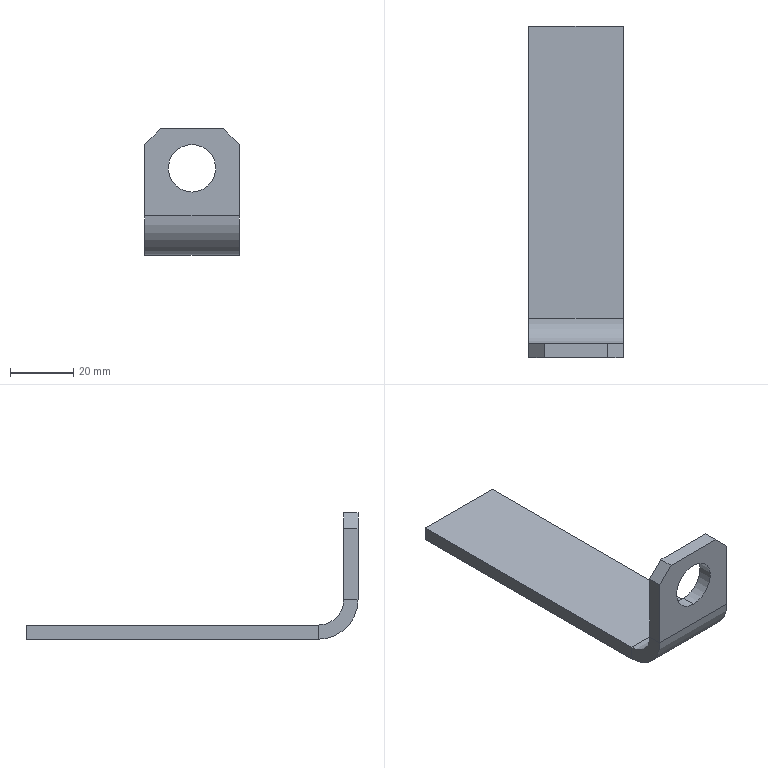Part | SolidWorks | features Chamfer 1, FlatPattern 1, ICE 1, SMBaseFlange 1, SheetMetal 1 | 1 solid | 18 faces | box 30 x 105 x 40 mm | volume 17466 mm3 | plane 14 | cylinder 4 | commonest cylinder face diameters 15 x2 16 x1 25 x1
STEP:
#1=CARTESIAN_POINT('',(0.,0.,-5.));
#2=VERTEX_POINT('',#1);
#3=CARTESIAN_POINT('',(0.,0.,-20.));
#4=VERTEX_POINT('',#3);
#5=CARTESIAN_POINT('',(0.,0.,-12.5));
#6=DIRECTION('',(0.,-1.,0.));
#7=DIRECTION('',(0.,0.,1.));
#8=AXIS2_PLACEMENT_3D('',#5,#6,#7);
#9=CIRCLE('',#8,7.5);
#10=EDGE_CURVE('',#2,#4,#9,.T.);
#11=ORIENTED_EDGE('',*,*,#10,.T.);
#12=CARTESIAN_POINT('',(0.,4.5,-20.));
#13=VERTEX_POINT('',#12);
#14=CARTESIAN_POINT('',(0.,-0.001,-20.));
#15=DIRECTION('',(0.,1.,0.));
#16=VECTOR('',#15,1000.);
#17=LINE('',#14,#16);
#18=EDGE_CURVE('',#4,#13,#17,.T.);
#19=ORIENTED_EDGE('',*,*,#18,.T.);
#20=CARTESIAN_POINT('',(0.,4.5,-5.));
#21=VERTEX_POINT('',#20);
#22=CARTESIAN_POINT('',(0.,4.5,-12.5));
#23=DIRECTION('',(0.,1.,0.));
#24=DIRECTION('',(0.,0.,1.));
#25=AXIS2_PLACEMENT_3D('',#22,#23,#24);
#26=CIRCLE('',#25,7.5);
#27=EDGE_CURVE('',#13,#21,#26,.T.);
#28=ORIENTED_EDGE('',*,*,#27,.T.);
#29=CARTESIAN_POINT('',(0.,-0.001,-5.));
#30=DIRECTION('',(0.,1.,0.));
#31=VECTOR('',#30,1000.);
#32=LINE('',#29,#31);
#33=EDGE_CURVE('',#2,#21,#32,.T.);
#34=ORIENTED_EDGE('',*,*,#33,.F.);
#35=EDGE_LOOP('',(#11,#19,#28,#34));
#36=FACE_OUTER_BOUND('',#35,.T.);
#37=CARTESIAN_POINT('',(0.,-0.001,-12.5));
#38=DIRECTION('',(0.,1.,0.));
#39=DIRECTION('',(0.,0.,1.));
#40=AXIS2_PLACEMENT_3D('',#37,#38,#39);
#41=CYLINDRICAL_SURFACE('',#40,7.5);
#42=ADVANCED_FACE('',(#36),#41,.F.);
#43=CARTESIAN_POINT('',(15.,0.,-27.5));
#44=VERTEX_POINT('',#43);
#45=CARTESIAN_POINT('',(15.,4.5,-27.5));
#46=VERTEX_POINT('',#45);
#47=CARTESIAN_POINT('',(15.,0.,-27.5));
#48=DIRECTION('',(0.,1.,0.));
#49=VECTOR('',#48,1000.);
#50=LINE('',#47,#49);
#51=EDGE_CURVE('',#44,#46,#50,.T.);
#52=ORIENTED_EDGE('',*,*,#51,.F.);
#53=CARTESIAN_POINT('',(15.,12.5,-40.));
#54=VERTEX_POINT('',#53);
#55=CARTESIAN_POINT('',(15.,12.5,-27.5));
#56=DIRECTION('',(1.,0.,0.));
#57=DIRECTION('',(0.,0.,1.));
#58=AXIS2_PLACEMENT_3D('',#55,#56,#57);
#59=CIRCLE('',#58,12.5);
#60=EDGE_CURVE('',#44,#54,#59,.T.);
#61=ORIENTED_EDGE('',*,*,#60,.T.);
#62=CARTESIAN_POINT('',(15.,12.5,-35.5));
#63=VERTEX_POINT('',#62);
#64=CARTESIAN_POINT('',(15.,12.5,-35.5));
#65=DIRECTION('',(0.,0.,-1.));
#66=VECTOR('',#65,1000.);
#67=LINE('',#64,#66);
#68=EDGE_CURVE('',#63,#54,#67,.T.);
#69=ORIENTED_EDGE('',*,*,#68,.F.);
#70=CARTESIAN_POINT('',(15.,12.5,-27.5));
#71=DIRECTION('',(1.,0.,0.));
#72=DIRECTION('',(0.,0.,-1.));
#73=AXIS2_PLACEMENT_3D('',#70,#71,#72);
#74=CIRCLE('',#73,8.);
#75=EDGE_CURVE('',#46,#63,#74,.T.);
#76=ORIENTED_EDGE('',*,*,#75,.F.);
#77=EDGE_LOOP('',(#52,#61,#69,#76));
#78=FACE_OUTER_BOUND('',#77,.T.);
#79=CARTESIAN_POINT('',(15.,0.,-27.5));
#80=DIRECTION('',(1.,0.,0.));
#81=DIRECTION('',(0.,0.,-1.));
#82=AXIS2_PLACEMENT_3D('',#79,#80,#81);
#83=PLANE('',#82);
#84=ADVANCED_FACE('',(#78),#83,.T.);
#85=CARTESIAN_POINT('',(15.,4.5,-5.));
#86=VERTEX_POINT('',#85);
#87=CARTESIAN_POINT('',(15.,4.5,0.));
#88=DIRECTION('',(0.,0.,-1.));
#89=VECTOR('',#88,1000.);
#90=LINE('',#87,#89);
#91=EDGE_CURVE('',#86,#46,#90,.T.);
#92=ORIENTED_EDGE('',*,*,#91,.F.);
#93=CARTESIAN_POINT('',(15.,0.,-5.));
#94=VERTEX_POINT('',#93);
#95=CARTESIAN_POINT('',(15.,12.5,-5.));
#96=DIRECTION('',(0.,-1.,0.));
#97=VECTOR('',#96,1000.);
#98=LINE('',#95,#97);
#99=EDGE_CURVE('',#86,#94,#98,.T.);
#100=ORIENTED_EDGE('',*,*,#99,.T.);
#101=CARTESIAN_POINT('',(15.,0.,0.));
#102=DIRECTION('',(0.,0.,-1.));
#103=VECTOR('',#102,1000.);
#104=LINE('',#101,#103);
#105=EDGE_CURVE('',#94,#44,#104,.T.);
#106=ORIENTED_EDGE('',*,*,#105,.T.);
#107=ORIENTED_EDGE('',*,*,#51,.T.);
#108=EDGE_LOOP('',(#92,#100,#106,#107));
#109=FACE_OUTER_BOUND('',#108,.T.);
#110=CARTESIAN_POINT('',(15.,12.5,-35.5));
#111=DIRECTION('',(1.,0.,0.));
#112=DIRECTION('',(0.,0.,-1.));
#113=AXIS2_PLACEMENT_3D('',#110,#111,#112);
#114=PLANE('',#113);
#115=ADVANCED_FACE('',(#109),#114,.T.);
#116=CARTESIAN_POINT('',(-15.,12.5,-40.));
#117=VERTEX_POINT('',#116);
#118=CARTESIAN_POINT('',(-15.,12.5,-35.5));
#119=VERTEX_POINT('',#118);
#120=CARTESIAN_POINT('',(-15.,12.5,-40.));
#121=DIRECTION('',(0.,0.,1.));
#122=VECTOR('',#121,1000.);
#123=LINE('',#120,#122);
#124=EDGE_CURVE('',#117,#119,#123,.T.);
#125=ORIENTED_EDGE('',*,*,#124,.F.);
#126=CARTESIAN_POINT('',(-15.,0.,-27.5));
#127=VERTEX_POINT('',#126);
#128=CARTESIAN_POINT('',(-15.,12.5,-27.5));
#129=DIRECTION('',(1.,0.,0.));
#130=DIRECTION('',(0.,0.,1.));
#131=AXIS2_PLACEMENT_3D('',#128,#129,#130);
#132=CIRCLE('',#131,12.5);
#133=EDGE_CURVE('',#127,#117,#132,.T.);
#134=ORIENTED_EDGE('',*,*,#133,.F.);
#135=CARTESIAN_POINT('',(-15.,4.5,-27.5));
#136=VERTEX_POINT('',#135);
#137=CARTESIAN_POINT('',(-15.,4.5,-27.5));
#138=DIRECTION('',(0.,-1.,0.));
#139=VECTOR('',#138,1000.);
#140=LINE('',#137,#139);
#141=EDGE_CURVE('',#136,#127,#140,.T.);
#142=ORIENTED_EDGE('',*,*,#141,.F.);
#143=CARTESIAN_POINT('',(-15.,12.5,-27.5));
#144=DIRECTION('',(1.,0.,0.));
#145=DIRECTION('',(0.,0.,-1.));
#146=AXIS2_PLACEMENT_3D('',#143,#144,#145);
#147=CIRCLE('',#146,8.);
#148=EDGE_CURVE('',#136,#119,#147,.T.);
#149=ORIENTED_EDGE('',*,*,#148,.T.);
#150=EDGE_LOOP('',(#125,#134,#142,#149));
#151=FACE_OUTER_BOUND('',#150,.T.);
#152=CARTESIAN_POINT('',(-15.,12.5,-40.));
#153=DIRECTION('',(-1.,0.,0.));
#154=DIRECTION('',(0.,0.,1.));
#155=AXIS2_PLACEMENT_3D('',#152,#153,#154);
#156=PLANE('',#155);
#157=ADVANCED_FACE('',(#151),#156,.T.);
#158=CARTESIAN_POINT('',(-15.,105.,-40.));
#159=VERTEX_POINT('',#158);
#160=CARTESIAN_POINT('',(-15.,0.,-40.));
#161=DIRECTION('',(0.,1.,0.));
#162=VECTOR('',#161,1000.);
#163=LINE('',#160,#162);
#164=EDGE_CURVE('',#117,#159,#163,.T.);
#165=ORIENTED_EDGE('',*,*,#164,.F.);
#166=ORIENTED_EDGE('',*,*,#124,.T.);
#167=CARTESIAN_POINT('',(-15.,105.,-35.5));
#168=VERTEX_POINT('',#167);
#169=CARTESIAN_POINT('',(-15.,0.,-35.5));
#170=DIRECTION('',(0.,1.,0.));
#171=VECTOR('',#170,1000.);
#172=LINE('',#169,#171);
#173=EDGE_CURVE('',#119,#168,#172,.T.);
#174=ORIENTED_EDGE('',*,*,#173,.T.);
#175=CARTESIAN_POINT('',(-15.,105.,-35.5));
#176=DIRECTION('',(0.,0.,-1.));
#177=VECTOR('',#176,1000.);
#178=LINE('',#175,#177);
#179=EDGE_CURVE('',#168,#159,#178,.T.);
#180=ORIENTED_EDGE('',*,*,#179,.T.);
#181=EDGE_LOOP('',(#165,#166,#174,#180));
#182=FACE_OUTER_BOUND('',#181,.T.);
#183=CARTESIAN_POINT('',(-15.,4.5,-27.5));
#184=DIRECTION('',(-1.,0.,0.));
#185=DIRECTION('',(0.,0.,1.));
#186=AXIS2_PLACEMENT_3D('',#183,#184,#185);
#187=PLANE('',#186);
#188=ADVANCED_FACE('',(#182),#187,.T.);
#189=ORIENTED_EDGE('',*,*,#164,.T.);
#190=CARTESIAN_POINT('',(15.,105.,-40.));
#191=VERTEX_POINT('',#190);
#192=CARTESIAN_POINT('',(15.,105.,-40.));
#193=DIRECTION('',(-1.,0.,0.));
#194=VECTOR('',#193,1000.);
#195=LINE('',#192,#194);
#196=EDGE_CURVE('',#191,#159,#195,.T.);
#197=ORIENTED_EDGE('',*,*,#196,.F.);
#198=CARTESIAN_POINT('',(15.,0.,-40.));
#199=DIRECTION('',(0.,1.,0.));
#200=VECTOR('',#199,1000.);
#201=LINE('',#198,#200);
#202=EDGE_CURVE('',#54,#191,#201,.T.);
#203=ORIENTED_EDGE('',*,*,#202,.F.);
#204=CARTESIAN_POINT('',(15.,12.5,-40.));
#205=DIRECTION('',(-1.,0.,0.));
#206=VECTOR('',#205,1000.);
#207=LINE('',#204,#206);
#208=EDGE_CURVE('',#54,#117,#207,.T.);
#209=ORIENTED_EDGE('',*,*,#208,.T.);
#210=EDGE_LOOP('',(#189,#197,#203,#209));
#211=FACE_OUTER_BOUND('',#210,.T.);
#212=CARTESIAN_POINT('',(15.,0.,-40.));
#213=DIRECTION('',(0.,0.,1.));
#214=DIRECTION('',(1.,0.,0.));
#215=AXIS2_PLACEMENT_3D('',#212,#213,#214);
#216=PLANE('',#215);
#217=ADVANCED_FACE('',(#211),#216,.F.);
#218=ORIENTED_EDGE('',*,*,#179,.F.);
#219=CARTESIAN_POINT('',(15.,105.,-35.5));
#220=VERTEX_POINT('',#219);
#221=CARTESIAN_POINT('',(15.,105.,-35.5));
#222=DIRECTION('',(-1.,0.,0.));
#223=VECTOR('',#222,1000.);
#224=LINE('',#221,#223);
#225=EDGE_CURVE('',#220,#168,#224,.T.);
#226=ORIENTED_EDGE('',*,*,#225,.F.);
#227=CARTESIAN_POINT('',(15.,105.,-35.5));
#228=DIRECTION('',(0.,0.,-1.));
#229=VECTOR('',#228,1000.);
#230=LINE('',#227,#229);
#231=EDGE_CURVE('',#220,#191,#230,.T.);
#232=ORIENTED_EDGE('',*,*,#231,.T.);
#233=ORIENTED_EDGE('',*,*,#196,.T.);
#234=EDGE_LOOP('',(#218,#226,#232,#233));
#235=FACE_OUTER_BOUND('',#234,.T.);
#236=CARTESIAN_POINT('',(15.,105.,-35.5));
#237=DIRECTION('',(0.,1.,0.));
#238=DIRECTION('',(0.,0.,1.));
#239=AXIS2_PLACEMENT_3D('',#236,#237,#238);
#240=PLANE('',#239);
#241=ADVANCED_FACE('',(#235),#240,.T.);
#242=ORIENTED_EDGE('',*,*,#173,.F.);
#243=CARTESIAN_POINT('',(15.,12.5,-35.5));
#244=DIRECTION('',(-1.,0.,0.));
#245=VECTOR('',#244,1000.);
#246=LINE('',#243,#245);
#247=EDGE_CURVE('',#63,#119,#246,.T.);
#248=ORIENTED_EDGE('',*,*,#247,.F.);
#249=CARTESIAN_POINT('',(15.,0.,-35.5));
#250=DIRECTION('',(0.,1.,0.));
#251=VECTOR('',#250,1000.);
#252=LINE('',#249,#251);
#253=EDGE_CURVE('',#63,#220,#252,.T.);
#254=ORIENTED_EDGE('',*,*,#253,.T.);
#255=ORIENTED_EDGE('',*,*,#225,.T.);
#256=EDGE_LOOP('',(#242,#248,#254,#255));
#257=FACE_OUTER_BOUND('',#256,.T.);
#258=CARTESIAN_POINT('',(15.,0.,-35.5));
#259=DIRECTION('',(0.,0.,1.));
#260=DIRECTION('',(1.,0.,0.));
#261=AXIS2_PLACEMENT_3D('',#258,#259,#260);
#262=PLANE('',#261);
#263=ADVANCED_FACE('',(#257),#262,.T.);
#264=ORIENTED_EDGE('',*,*,#148,.F.);
#265=CARTESIAN_POINT('',(15.,4.5,-27.5));
#266=DIRECTION('',(-1.,0.,0.));
#267=VECTOR('',#266,1000.);
#268=LINE('',#265,#267);
#269=EDGE_CURVE('',#46,#136,#268,.T.);
#270=ORIENTED_EDGE('',*,*,#269,.F.);
#271=ORIENTED_EDGE('',*,*,#75,.T.);
#272=ORIENTED_EDGE('',*,*,#247,.T.);
#273=EDGE_LOOP('',(#264,#270,#271,#272));
#274=FACE_OUTER_BOUND('',#273,.T.);
#275=CARTESIAN_POINT('',(15.,12.5,-27.5));
#276=DIRECTION('',(-1.,0.,0.));
#277=DIRECTION('',(0.,0.,1.));
#278=AXIS2_PLACEMENT_3D('',#275,#276,#277);
#279=CYLINDRICAL_SURFACE('',#278,8.);
#280=ADVANCED_FACE('',(#274),#279,.F.);
#281=CARTESIAN_POINT('',(0.,4.5,-12.5));
#282=DIRECTION('',(0.,1.,0.));
#283=DIRECTION('',(0.,0.,1.));
#284=AXIS2_PLACEMENT_3D('',#281,#282,#283);
#285=CIRCLE('',#284,7.5);
#286=EDGE_CURVE('',#21,#13,#285,.T.);
#287=ORIENTED_EDGE('',*,*,#286,.F.);
#288=ORIENTED_EDGE('',*,*,#27,.F.);
#289=EDGE_LOOP('',(#287,#288));
#290=FACE_BOUND('',#289,.T.);
#291=CARTESIAN_POINT('',(-15.,4.5,-5.));
#292=VERTEX_POINT('',#291);
#293=CARTESIAN_POINT('',(-15.,4.5,0.));
#294=DIRECTION('',(0.,0.,-1.));
#295=VECTOR('',#294,1000.);
#296=LINE('',#293,#295);
#297=EDGE_CURVE('',#292,#136,#296,.T.);
#298=ORIENTED_EDGE('',*,*,#297,.F.);
#299=CARTESIAN_POINT('',(-10.,4.5,0.));
#300=VERTEX_POINT('',#299);
#301=CARTESIAN_POINT('',(2.5,4.5,12.5));
#302=DIRECTION('',(0.7071,0.,0.7071));
#303=VECTOR('',#302,1000.);
#304=LINE('',#301,#303);
#305=EDGE_CURVE('',#292,#300,#304,.T.);
#306=ORIENTED_EDGE('',*,*,#305,.T.);
#307=CARTESIAN_POINT('',(10.,4.5,0.));
#308=VERTEX_POINT('',#307);
#309=CARTESIAN_POINT('',(15.,4.5,0.));
#310=DIRECTION('',(-1.,0.,0.));
#311=VECTOR('',#310,1000.);
#312=LINE('',#309,#311);
#313=EDGE_CURVE('',#308,#300,#312,.T.);
#314=ORIENTED_EDGE('',*,*,#313,.F.);
#315=CARTESIAN_POINT('',(12.5,4.5,-2.5));
#316=DIRECTION('',(0.7071,0.,-0.7071));
#317=VECTOR('',#316,1000.);
#318=LINE('',#315,#317);
#319=EDGE_CURVE('',#308,#86,#318,.T.);
#320=ORIENTED_EDGE('',*,*,#319,.T.);
#321=ORIENTED_EDGE('',*,*,#91,.T.);
#322=ORIENTED_EDGE('',*,*,#269,.T.);
#323=EDGE_LOOP('',(#298,#306,#314,#320,#321,#322));
#324=FACE_OUTER_BOUND('',#323,.T.);
#325=CARTESIAN_POINT('',(15.,4.5,0.));
#326=DIRECTION('',(0.,1.,0.));
#327=DIRECTION('',(0.,0.,1.));
#328=AXIS2_PLACEMENT_3D('',#325,#326,#327);
#329=PLANE('',#328);
#330=ADVANCED_FACE('',(#290,#324),#329,.T.);
#331=ORIENTED_EDGE('',*,*,#313,.T.);
#332=CARTESIAN_POINT('',(-10.,0.,0.));
#333=VERTEX_POINT('',#332);
#334=CARTESIAN_POINT('',(-10.,0.,0.));
#335=DIRECTION('',(0.,-1.,0.));
#336=VECTOR('',#335,1000.);
#337=LINE('',#334,#336);
#338=EDGE_CURVE('',#300,#333,#337,.T.);
#339=ORIENTED_EDGE('',*,*,#338,.T.);
#340=CARTESIAN_POINT('',(10.,0.,0.));
#341=VERTEX_POINT('',#340);
#342=CARTESIAN_POINT('',(15.,0.,0.));
#343=DIRECTION('',(-1.,0.,0.));
#344=VECTOR('',#343,1000.);
#345=LINE('',#342,#344);
#346=EDGE_CURVE('',#341,#333,#345,.T.);
#347=ORIENTED_EDGE('',*,*,#346,.F.);
#348=CARTESIAN_POINT('',(10.,0.,0.));
#349=DIRECTION('',(0.,1.,0.));
#350=VECTOR('',#349,1000.);
#351=LINE('',#348,#350);
#352=EDGE_CURVE('',#341,#308,#351,.T.);
#353=ORIENTED_EDGE('',*,*,#352,.T.);
#354=EDGE_LOOP('',(#331,#339,#347,#353));
#355=FACE_OUTER_BOUND('',#354,.T.);
#356=CARTESIAN_POINT('',(15.,0.,0.));
#357=DIRECTION('',(0.,0.,1.));
#358=DIRECTION('',(1.,0.,0.));
#359=AXIS2_PLACEMENT_3D('',#356,#357,#358);
#360=PLANE('',#359);
#361=ADVANCED_FACE('',(#355),#360,.T.);
#362=ORIENTED_EDGE('',*,*,#10,.F.);
#363=CARTESIAN_POINT('',(0.,0.,-12.5));
#364=DIRECTION('',(0.,-1.,0.));
#365=DIRECTION('',(0.,0.,1.));
#366=AXIS2_PLACEMENT_3D('',#363,#364,#365);
#367=CIRCLE('',#366,7.5);
#368=EDGE_CURVE('',#4,#2,#367,.T.);
#369=ORIENTED_EDGE('',*,*,#368,.F.);
#370=EDGE_LOOP('',(#362,#369));
#371=FACE_BOUND('',#370,.T.);
#372=ORIENTED_EDGE('',*,*,#346,.T.);
#373=CARTESIAN_POINT('',(-15.,0.,-5.));
#374=VERTEX_POINT('',#373);
#375=CARTESIAN_POINT('',(-15.,0.,-5.));
#376=DIRECTION('',(-0.7071,0.,-0.7071));
#377=VECTOR('',#376,1000.);
#378=LINE('',#375,#377);
#379=EDGE_CURVE('',#333,#374,#378,.T.);
#380=ORIENTED_EDGE('',*,*,#379,.T.);
#381=CARTESIAN_POINT('',(-15.,0.,0.));
#382=DIRECTION('',(0.,0.,-1.));
#383=VECTOR('',#382,1000.);
#384=LINE('',#381,#383);
#385=EDGE_CURVE('',#374,#127,#384,.T.);
#386=ORIENTED_EDGE('',*,*,#385,.T.);
#387=CARTESIAN_POINT('',(15.,0.,-27.5));
#388=DIRECTION('',(-1.,0.,0.));
#389=VECTOR('',#388,1000.);
#390=LINE('',#387,#389);
#391=EDGE_CURVE('',#44,#127,#390,.T.);
#392=ORIENTED_EDGE('',*,*,#391,.F.);
#393=ORIENTED_EDGE('',*,*,#105,.F.);
#394=CARTESIAN_POINT('',(10.,0.,0.));
#395=DIRECTION('',(-0.7071,0.,0.7071));
#396=VECTOR('',#395,1000.);
#397=LINE('',#394,#396);
#398=EDGE_CURVE('',#94,#341,#397,.T.);
#399=ORIENTED_EDGE('',*,*,#398,.T.);
#400=EDGE_LOOP('',(#372,#380,#386,#392,#393,#399));
#401=FACE_OUTER_BOUND('',#400,.T.);
#402=CARTESIAN_POINT('',(15.,0.,0.));
#403=DIRECTION('',(0.,1.,0.));
#404=DIRECTION('',(0.,0.,1.));
#405=AXIS2_PLACEMENT_3D('',#402,#403,#404);
#406=PLANE('',#405);
#407=ADVANCED_FACE('',(#371,#401),#406,.F.);
#408=ORIENTED_EDGE('',*,*,#133,.T.);
#409=ORIENTED_EDGE('',*,*,#208,.F.);
#410=ORIENTED_EDGE('',*,*,#60,.F.);
#411=ORIENTED_EDGE('',*,*,#391,.T.);
#412=EDGE_LOOP('',(#408,#409,#410,#411));
#413=FACE_OUTER_BOUND('',#412,.T.);
#414=CARTESIAN_POINT('',(15.,12.5,-27.5));
#415=DIRECTION('',(-1.,0.,0.));
#416=DIRECTION('',(0.,0.,1.));
#417=AXIS2_PLACEMENT_3D('',#414,#415,#416);
#418=CYLINDRICAL_SURFACE('',#417,12.5);
#419=ADVANCED_FACE('',(#413),#418,.T.);
#420=ORIENTED_EDGE('',*,*,#202,.T.);
#421=ORIENTED_EDGE('',*,*,#231,.F.);
#422=ORIENTED_EDGE('',*,*,#253,.F.);
#423=ORIENTED_EDGE('',*,*,#68,.T.);
#424=EDGE_LOOP('',(#420,#421,#422,#423));
#425=FACE_OUTER_BOUND('',#424,.T.);
#426=CARTESIAN_POINT('',(15.,12.5,-27.5));
#427=DIRECTION('',(1.,0.,0.));
#428=DIRECTION('',(0.,0.,-1.));
#429=AXIS2_PLACEMENT_3D('',#426,#427,#428);
#430=PLANE('',#429);
#431=ADVANCED_FACE('',(#425),#430,.T.);
#432=ORIENTED_EDGE('',*,*,#385,.F.);
#433=CARTESIAN_POINT('',(-15.,4.5,-5.));
#434=DIRECTION('',(0.,1.,0.));
#435=VECTOR('',#434,1000.);
#436=LINE('',#433,#435);
#437=EDGE_CURVE('',#374,#292,#436,.T.);
#438=ORIENTED_EDGE('',*,*,#437,.T.);
#439=ORIENTED_EDGE('',*,*,#297,.T.);
#440=ORIENTED_EDGE('',*,*,#141,.T.);
#441=EDGE_LOOP('',(#432,#438,#439,#440));
#442=FACE_OUTER_BOUND('',#441,.T.);
#443=CARTESIAN_POINT('',(-15.,12.5,-27.5));
#444=DIRECTION('',(1.,0.,0.));
#445=DIRECTION('',(0.,0.,-1.));
#446=AXIS2_PLACEMENT_3D('',#443,#444,#445);
#447=PLANE('',#446);
#448=ADVANCED_FACE('',(#442),#447,.F.);
#449=ORIENTED_EDGE('',*,*,#18,.F.);
#450=ORIENTED_EDGE('',*,*,#368,.T.);
#451=ORIENTED_EDGE('',*,*,#33,.T.);
#452=ORIENTED_EDGE('',*,*,#286,.T.);
#453=EDGE_LOOP('',(#449,#450,#451,#452));
#454=FACE_OUTER_BOUND('',#453,.T.);
#455=CARTESIAN_POINT('',(0.,-0.001,-12.5));
#456=DIRECTION('',(0.,1.,0.));
#457=DIRECTION('',(0.,0.,1.));
#458=AXIS2_PLACEMENT_3D('',#455,#456,#457);
#459=CYLINDRICAL_SURFACE('',#458,7.5);
#460=ADVANCED_FACE('',(#454),#459,.F.);
#461=ORIENTED_EDGE('',*,*,#379,.F.);
#462=ORIENTED_EDGE('',*,*,#338,.F.);
#463=ORIENTED_EDGE('',*,*,#305,.F.);
#464=ORIENTED_EDGE('',*,*,#437,.F.);
#465=EDGE_LOOP('',(#461,#462,#463,#464));
#466=FACE_OUTER_BOUND('',#465,.T.);
#467=CARTESIAN_POINT('',(-15.,12.5,-5.));
#468=DIRECTION('',(-0.7071,0.,0.7071));
#469=DIRECTION('',(0.,-1.,0.));
#470=AXIS2_PLACEMENT_3D('',#467,#468,#469);
#471=PLANE('',#470);
#472=ADVANCED_FACE('',(#466),#471,.T.);
#473=ORIENTED_EDGE('',*,*,#398,.F.);
#474=ORIENTED_EDGE('',*,*,#99,.F.);
#475=ORIENTED_EDGE('',*,*,#319,.F.);
#476=ORIENTED_EDGE('',*,*,#352,.F.);
#477=EDGE_LOOP('',(#473,#474,#475,#476));
#478=FACE_OUTER_BOUND('',#477,.T.);
#479=CARTESIAN_POINT('',(10.,0.,0.));
#480=DIRECTION('',(-0.7071,0.,-0.7071));
#481=DIRECTION('',(0.,1.,0.));
#482=AXIS2_PLACEMENT_3D('',#479,#480,#481);
#483=PLANE('',#482);
#484=ADVANCED_FACE('',(#478),#483,.F.);
#485=CLOSED_SHELL('',(#42,#84,#115,#157,#188,#217,#241,#263,#280,#330,#361,#407,#419,#431,#448,#460,#472,#484));
#486=MANIFOLD_SOLID_BREP('',#485);
#487=CARTESIAN_POINT('',(0.,0.,0.));
#488=DIRECTION('',(0.,0.,1.));
#489=DIRECTION('',(1.,0.,0.));
#490=AXIS2_PLACEMENT_3D('',#487,#488,#489);
#491=(LENGTH_UNIT()NAMED_UNIT(*)SI_UNIT(.MILLI.,.METRE.));
#492=UNCERTAINTY_MEASURE_WITH_UNIT(LENGTH_MEASURE(0.00001),#491,'','');
#493=(NAMED_UNIT(*)PLANE_ANGLE_UNIT()SI_UNIT($,.RADIAN.));
#494=(NAMED_UNIT(*)SI_UNIT($,.STERADIAN.)SOLID_ANGLE_UNIT());
#495=(GEOMETRIC_REPRESENTATION_CONTEXT(3)GLOBAL_UNCERTAINTY_ASSIGNED_CONTEXT((#492))GLOBAL_UNIT_ASSIGNED_CONTEXT((#491,#493,#494))REPRESENTATION_CONTEXT('',''));
#496=ADVANCED_BREP_SHAPE_REPRESENTATION('',(#486,#490),#495);